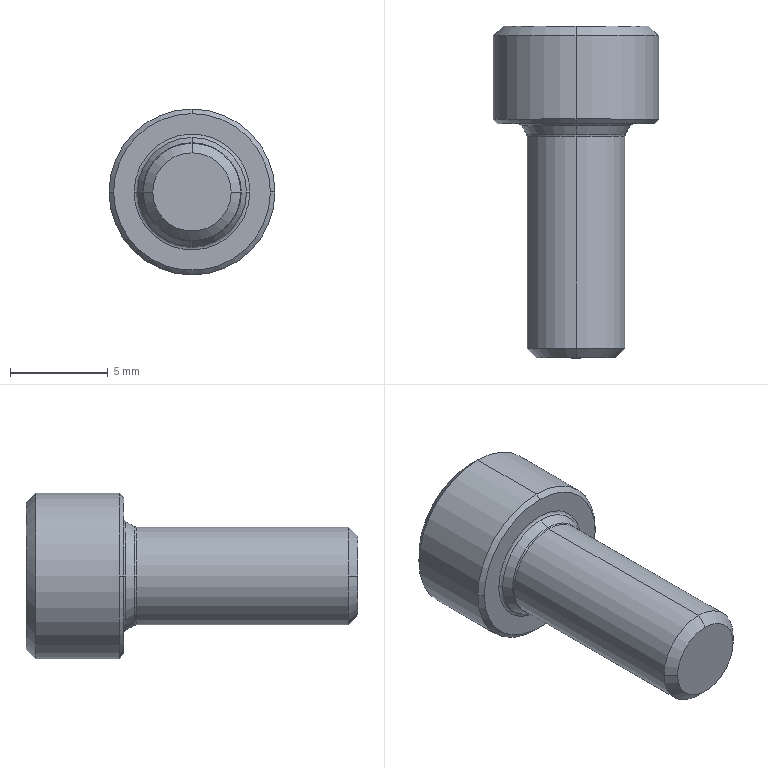Part | STEP file | 1 solid | 44 faces | box 8.5 x 17 x 8.5 mm | volume 468.205 mm3 | cone 19 | plane 15 | cylinder 6 | spline 4 | commonest cylinder face diameters 4 x2 5 x2 8.5 x2